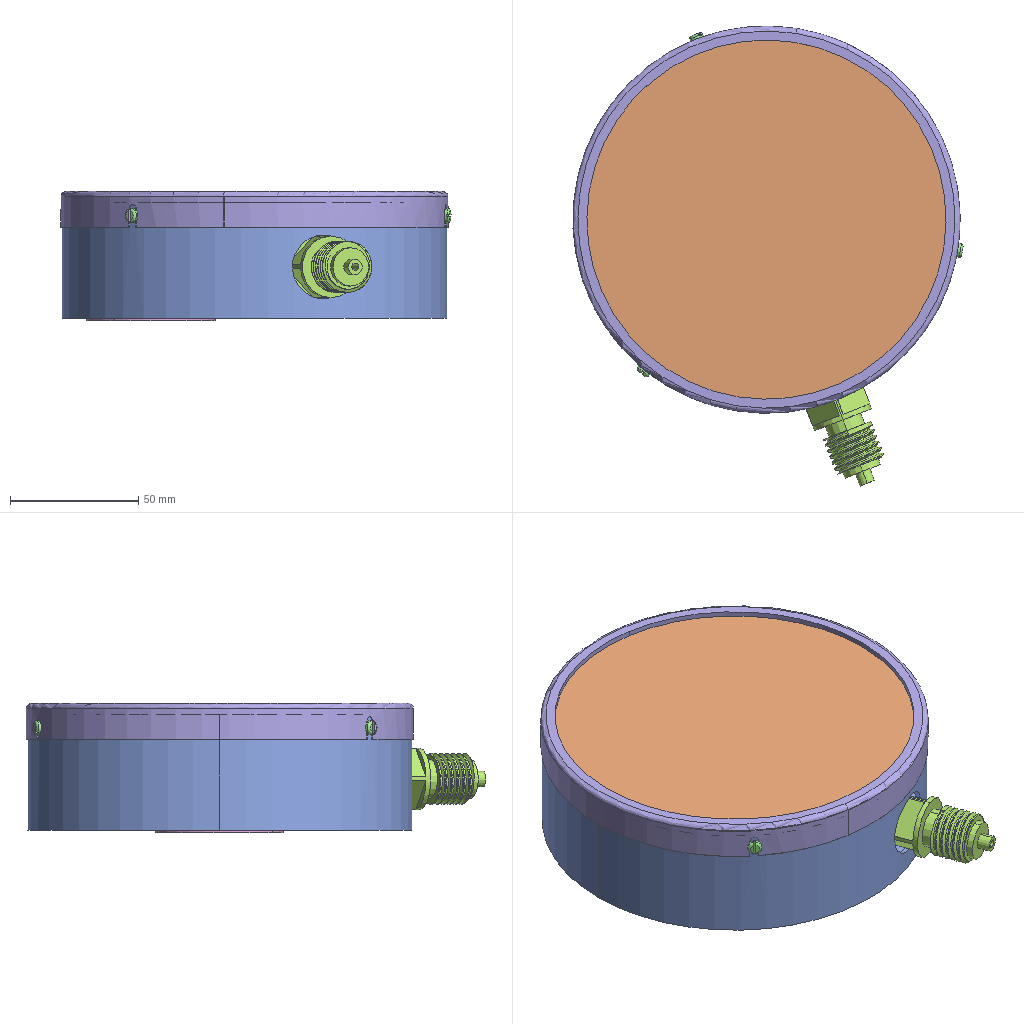Assembly | SolidWorks | 29 different items | 32 placed | box 152 x 179 x 51 mm
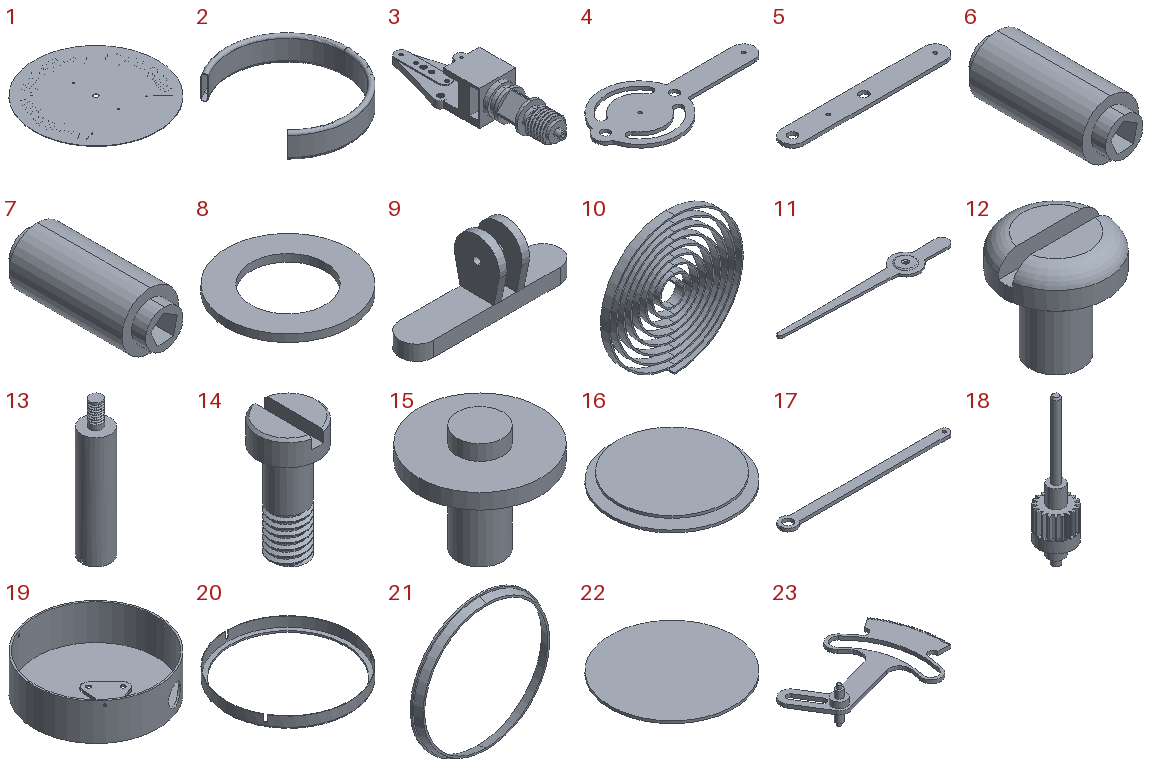Parts list (item | name | quantity | size | volume | features):
1 | - | x1 | 137 x 137 x 1 mm | 7784 mm3 | features ICE 5, CirPattern 2, Cut 1, Extrusion 1
2 | - | x1 | 93.293 x 109.3 x 21.3 mm | 3338 mm3 | features Sweep 1
3 | - | x1 | 35 x 140 x 30.32 mm | 37050 mm3 | features ICE 15, Helix 8, SweepCut 8, Cut 2, Chamfer 1, CirPattern 1, Extrusion 1
4 | - | x1 | 74 x 36 x 1.5 mm | 1679 mm3 | features Extrusion 1
5 | - | x1 | 74 x 10 x 1.5 mm | 1035 mm3 | features Extrusion 1
6 | - | x1 | 6 x 14.5 x 6 mm | 291.486 mm3 | features ICE 5, Extrusion 1
7 | - | x1 | 6 x 14.5 x 6 mm | 290.19 mm3 | features ICE 6, Extrusion 1
8 | - | x2 | 5 x 5 x 0.3 mm | 3.77 mm3 | features Extrusion 1, ICE 1
9 | - | x1 | 21.3 x 6 x 9 mm | 252.148 mm3 | features ICE 2, Extrusion 1
10 | - | x1 | 34.782 x 2.18 x 35.72 mm | 426.683 mm3 | features ExtruThin 1
11 | - | x1 | 74.73 x 12.196 x 3.5 mm | 394.358 mm3 | features ICE 4, Extrusion 1, Fillet 1
12 | - | x3 | 5.6 x 5.6 x 5.8 mm | 61.126 mm3 | features ICE 3, Revolution 2, Extrusion 1, RevCut 1
13 | - | x1 | 6 x 6 x 28 mm | 660.837 mm3 | features ICE 3, RevCut 2, Extrusion 1, Helix 1, RefAxis 1, SweepThread 1
14 | - | x1 | 5 x 5 x 10 mm | 85.863 mm3 | features ICE 2, Extrusion 1, Helix 1, RevCut 1, SweepCut 1
15 | - | x1 | 8 x 8 x 7 mm | 95.001 mm3 | features ICE 3, Extrusion 1, RevCut 1
16 | - | x1 | 50 x 50 x 4 mm | 5752 mm3 | features ICE 2, Extrusion 1
17 | - | x1 | 53.128 x 5 x 1 mm | 155.677 mm3 | features Extrusion 1
18 | - | x1 | 6.634 x 6.634 x 28 mm | 248.912 mm3 | features ICE 5, Extrusion 1, RefAxis 1, RevCut 1
19 | - | x1 | 150 x 150 x 45 mm | 73548 mm3 | features ICE 7, CirPattern 1, Cut 1, Extrusion 1, Fillet 1
20 | - | x1 | 151 x 151 x 14 mm | 7416 mm3 | features ICE 3, CirPattern 1, Extrusion 1, Fillet 1
21 | - | x1 | 148 x 10 x 148 mm | 10057 mm3 | features Revolution 1
22 | - | x1 | 148 x 148 x 3 mm | 51610 mm3 | features Extrusion 1
23 | - | x1 | 57.266 x 39.218 x 15 mm | 1123 mm3 | features ICE 6, Extrusion 1
24 | parallel pins hardening steel gb | x1 | - | - | -
25 | slotted cheese head screws gb | x1 | - | - | -
26 | slotted cheese head screws with shoulder gb | x1 | - | - | -
27 | slotted large raised cheese head screws gb | x1 | - | - | -
28 | slotted pan head screws gb | x1 | - | - | -
29 | small hex thin nuts-fine pitch thread gb | x1 | - | - | -
Mates (type | each side: item.copy, entity, surface, feature):
Coincident | 19.1 face plane Boss-Extrude 3 | 3.1 face plane Boss-Extrude 1
Parallel | 19.1 edge | 3.1 edge
Concentric | 19.1 edge | 3.1 edge
Concentric | 19.1 edge | 16.1 edge
Coincident | 19.1 face plane Cut-Extrude 10 | 16.1 face plane Boss-Extrude 1
Concentric | 3.1 edge | 13.1 edge
Coincident | 3.1 face plane Boss-Extrude 5 | 13.1 face plane Boss-Extrude 1
Coincident | 3.1 face plane Boss-Extrude 5 | 4.1 face plane Boss-Extrude 1
Concentric | 3.1 edge | 4.1 edge
LimitPlanarAngleDim | 4.1 face plane Boss-Extrude 1 | 3.1 face plane Boss-Extrude 1
Concentric | 4.1 edge | 18.1 edge
Coincident | 4.1 face plane Boss-Extrude 1 | 18.1 face plane Boss-Extrude 3
Concentric | 4.1 edge | 7.1 edge
Coincident | 4.1 face plane Boss-Extrude 1 | 7.1 face plane Boss-Extrude 3
Concentric | 4.1 edge | 6.1 edge
Coincident | 4.1 face plane Boss-Extrude 1 | 6.1 face plane Boss-Extrude 3
Coincident | 4.1 face plane Boss-Extrude 1 | 23.1 face plane Boss-Extrude 5
Concentric | 23.1 edge | 14.1 edge
Concentric | 17.1 edge | 14.1 edge
Coincident | 17.1 face plane Boss-Extrude 1 | 14.1 face plane Boss-Extrude 1
Concentric | 14.1 edge | 8.1 edge
Coincident | 17.1 face plane Boss-Extrude 1 | 8.1 face plane Boss-Extrude 1
Concentric | 8.1 edge | 8.2 edge
Coincident | 8.1 face plane Boss-Extrude 1 | 8.2 face plane Boss-Extrude 1
DistanceDim | 8.2 face plane Boss-Extrude 1 | 23.1 face plane Boss-Extrude 2
Coincident | 2.1 face plane Sweep 2 | 9.1 face plane Boss-Extrude 1
Concentric | 2.1 edge | 9.1 edge
Coincident | 2.1 edge | 9.1 edge
Concentric | 5.1 edge | 23.1 edge
Coincident | 23.1 face plane Boss-Extrude 7 | 5.1 face plane Boss-Extrude 1
Concentric | 18.1 edge | 5.1 edge
Concentric | 18.1 edge | 2.1 edge
Concentric | 1.1 edge | 3.1 edge
Concentric | 13.1 face cylinder Boss-Extrude 1 | 1.1 edge
Coincident | 3.1 face plane Boss-Extrude 1 | 1.1 face plane Boss-Extrude 1
Concentric | 11.1 edge | 18.1 edge
Coincident | 18.1 face plane Boss-Extrude 6 | 11.1 face plane Boss-Extrude 5
Concentric | 1.1 edge | 15.1 edge
Coincident | 1.1 face plane Boss-Extrude 1 | 15.1 face plane Boss-Extrude 2
Concentric | 19.1 edge | 22.1 edge
Concentric | 19.1 edge | 21.1 edge
Coincident | 1.1 face plane Boss-Extrude 1 | 21.1 face plane Revolve 1
Coincident | 21.1 face plane Revolve 1 | 22.1 face plane Boss-Extrude 1
Coincident | 22.1 face plane Boss-Extrude 1 | 20.1 face plane Boss-Extrude 2
Concentric | 21.1 edge | 20.1 edge
Concentric | 19.1 face cylinder Circular pattern 1 | 12.1 face cylinder Boss-Extrude 3
Tangent | 20.1 face cylinder Boss-Extrude 1 | 12.1 face plane Boss-Extrude 1
Concentric | 19.1 face cylinder Cut-Extrude 22 | 12.2 face cylinder Boss-Extrude 3
Tangent | 20.1 face cylinder Boss-Extrude 1 | 12.2 face plane Boss-Extrude 1
Concentric | 19.1 face cylinder Circular pattern 1 | 12.3 face cylinder Boss-Extrude 3
Tangent | 20.1 face cylinder Boss-Extrude 1 | 12.3 face plane Boss-Extrude 1
Lock | 19.1 select_type:0 | 2.1 select_type:0
GearDim | 18.1 face cylinder Boss-Extrude 1 | 23.1 face cylinder Boss-Extrude 2
Concentric | 18.1 edge | 10.1 edge
Coincident | 18.1 face plane Boss-Extrude 2 | 10.1 face plane Extrude-thin 2